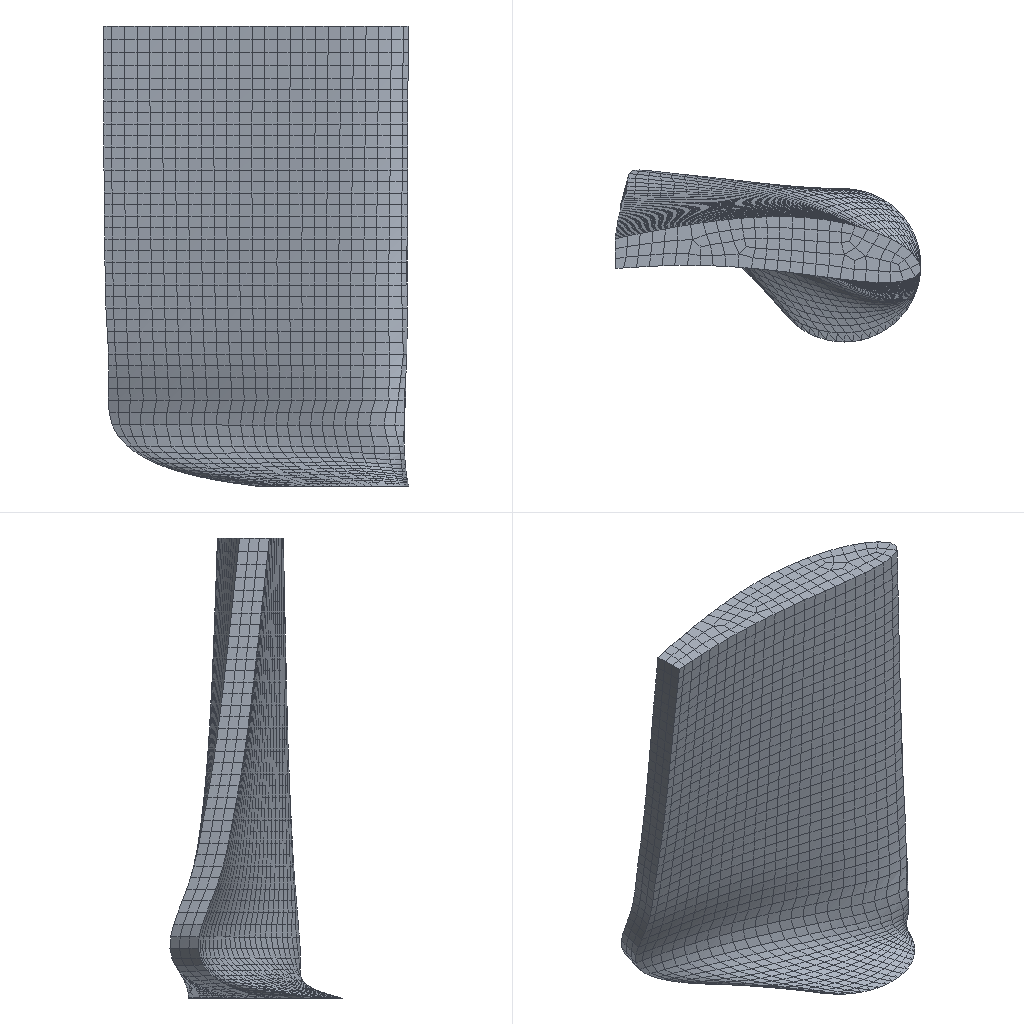Simulation study | abaqus
Set-up summary:
category,name,step,type,value,unit,region
solver,abaqus,,Abaqus/CAE 2024
units,SI m-kg-s (Pa),,inferred,E=1.5e+10 density=900
analysis,Step-1,,dynamic explicit,nlgeom=True; time_period=2.218
mesh,nodes,,,6429
mesh,elements,,,4944
element_type,C3D8R,,,4944
material,WOOD,,E,1.5e+10
material,WOOD,,nu,0.3
material,WOOD,,density,900
material,WOOD,,behaviors,damping
section,WOOD,,solid section,,,Set-1
load,Q1,Step-1,concentrated force,"1 [dir=(1, 0, 0)]",,Set-1
load,Q2,Step-1,concentrated force,"1 [dir=(1, 0, 0)]",,Set-2
load,Q3,Step-1,concentrated force,"1 [dir=(1, 0, 0)]",,Set-3
load,Q4,Step-1,concentrated force,"1 [dir=(1, 0, 0)]",,Set-4
load,Q5,Step-1,concentrated force,"1 [dir=(1, 0, 0)]",,Set-5
load,Q6,Step-1,concentrated force,"1 [dir=(1, 0, 0)]",,Set-6
load,Q7,Step-1,concentrated force,"1 [dir=(1, 0, 0)]",,Set-7
load,Q8,Step-1,concentrated force,"1 [dir=(1, 0, 0)]",,Set-8
load,Q9,Step-1,concentrated force,"1 [dir=(1, 0, 0)]",,Set-9
load,Q10,Step-1,concentrated force,"1 [dir=(1, 0, 0)]",,Set-10
load,Z1,Step-1,concentrated force,"1 [dir=(0, 1, 0)]",,Set-1
load,Z2,Step-1,concentrated force,"1 [dir=(0, 1, 0)]",,Set-2
load,Z3,Step-1,concentrated force,"1 [dir=(0, 1, 0)]",,Set-3
load,Z4,Step-1,concentrated force,"1 [dir=(0, 1, 0)]",,Set-4
load,Z5,Step-1,concentrated force,"1 [dir=(0, 1, 0)]",,Set-5
load,Z6,Step-1,concentrated force,"1 [dir=(0, 1, 0)]",,Set-6
load,Z7,Step-1,concentrated force,"1 [dir=(0, 1, 0)]",,Set-7
load,Z8,Step-1,concentrated force,"1 [dir=(0, 1, 0)]",,Set-8
load,Z9,Step-1,concentrated force,"1 [dir=(0, 1, 0)]",,Set-9
load,Z10,Step-1,concentrated force,"1 [dir=(0, 1, 0)]",,Set-10
bc,BC-1,Step-1,encastre,[dofs=ENCASTRE],,_PickedSet47
Abaqus input file, long lists of numbers shortened, first 290 of 1023 lines:
*Heading
** Job name: deck Model name: Model-1-Copy-Copy
** Generated by: Abaqus/CAE 2024
*Preprint, echo=NO, model=NO, history=NO, contact=NO
**
** PARTS
**
*Part, name=P16CMblade-Copy
*End Part
**
**
** ASSEMBLY
**
*Assembly, name=Assembly
**
*Instance, name=P16CMblade-Copy-1, part=P16CMblade-Copy
*Node
      1, -0.3723,  0.05119,  0.8526
      2, -0.3725, 0.002756,  0.8526
** (6417 more lines like these left out)
*Element, type=C3D8R
  1,    2,   26,  671,   27,   77,  975, 3494,  874
  2,   75,  698,  744,   76,  826, 3521, 3567,  825
** (4942 more lines like these left out)
*Nset, nset=Set-1, generate
    1,  6419,     1
*Elset, elset=Set-1, generate
    1,  4944,     1
** Section: Section-1
*Solid Section, elset=Set-1, material=WOOD
,
*End Instance
**
*Node
      1, -0.06243, 0.04167,  0.2223
*Node
      2, -0.09256, 0.05414,  0.2991
*Node
      3, -0.09701, 0.04794,  0.3745
*Node
      4, -0.1035, 0.045,  0.4497
*Node
      5, -0.108, 0.04136,  0.5244
*Node
      6, -0.1074,  0.03725,  0.6
*Node
      7, -0.106, 0.03382,  0.6742
*Node
      8, -0.1069, 0.03147,  0.7492
*Node
      9, -0.1111, 0.02943,  0.8249
*Node
     10, -0.1145, 0.02727,  0.8996
*Nset, nset=Set-1, instance=P16CMblade-Copy-1
 2706,
*Nset, nset=Set-2, instance=P16CMblade-Copy-1
 2423,
*Nset, nset=Set-3, instance=P16CMblade-Copy-1
 2190,
*Nset, nset=Set-4, instance=P16CMblade-Copy-1
 1957,
*Nset, nset=Set-5, instance=P16CMblade-Copy-1
 1725,
*Nset, nset=Set-6, instance=P16CMblade-Copy-1
 1535,
*Nset, nset=Set-7, instance=P16CMblade-Copy-1
 4057,
*Nset, nset=Set-8, instance=P16CMblade-Copy-1
 1119,
*Nset, nset=Set-9, instance=P16CMblade-Copy-1
 3595,
*Nset, nset=Set-10, instance=P16CMblade-Copy-1
 3376,
*Nset, nset=_PickedSet47, internal, instance=P16CMblade-Copy-1
   19,   20,   21,   22,  552,  553,  554,  555,  556,  557,  558,  559,  560,  561,  562,  563
  564,  565,  566,  567,  568,  569,  570,  571,  572,  573,  574,  575,  576,  577,  578,  579
** (7 more lines like these left out)
*Elset, elset=_PickedSet47, internal, instance=P16CMblade-Copy-1, generate
 4430,  4532,     1
*End Assembly
*Amplitude, name=Q1
          0.001,     0.0008927,           0.002,    -10.208,           0.003,    -15.004,           0.004,    -14.992
          0.005,    -14.896,           0.006,    -14.758,           0.007,    -14.573,           0.008,    -14.344
          0.009,    -14.078,            0.01,    -13.783,           0.011,    -13.456,           0.012,       -13.104
          0.013,    -12.739,           0.014,    -12.363,           0.015,    -11.999,           0.016,    -11.648
          0.017,    -11.318,           0.018,    -10.972,           0.019,    -10.59,            0.02,    -10.166
          0.021,    -9.717,           0.022,    -9.265,           0.023,    -8.835,           0.024,    -8.422
          0.025,    -8.028,           0.026,    -7.64,           0.027,    -7.247,           0.028,    -6.843
          0.029,    -6.429,            0.03,    -6.017,           0.031,    -5.621,           0.032,    -5.255
          0.033,    -4.946,           0.034,        -4.699,           0.035,    -4.522,           0.036,    -4.407
          0.037,    -4.336,           0.038,       -4.284,           0.039,    -4.228,            0.04,    -4.158
          0.041,    -4.061,           0.042,    -3.941,           0.043,    -3.805,           0.044,    -3.664
          0.045,    -3.439,           0.046,    -3.417,           0.047,         -3.45,           0.048,    -3.538
          0.049,    -3.663,            0.05,       -3.821,           0.051,       -4.012,           0.052,    -4.231
          0.053,    -4.472,           0.054,    -4.724,           0.055,    -4.957,           0.056,    -5.158
          0.057,    -5.33,           0.058,    -5.464,           0.059,    -5.548,            0.06,        -5.586
          0.061,    -5.589,           0.062,        -5.557,           0.063,    -5.501,           0.064,    -5.431
          0.065,    -5.347,           0.066,    -5.25,           0.067,    -5.13,           0.068,    -4.986
          0.069,    -4.816,            0.07,    -4.623,           0.071,    -4.417,           0.072,       -4.213
          0.073,    -4.034,           0.074,    -3.895,           0.075,    -3.803,           0.076,    -3.761
          0.077,    -3.761,           0.078,    -3.785,           0.079,    -3.831,            0.08,    -3.893
          0.081,    -3.96,           0.082,    -4.025,           0.083,    -4.081,           0.084,    -4.123
          0.085,        -4.149,           0.086,       -4.165,           0.087,    -4.17,           0.088,    -4.169
          0.089,       -4.161,            0.09,    -4.144,           0.091,    -4.125,           0.092,    -4.095
          0.093,    -4.052,           0.094,    -4.,           0.095,    -3.945,           0.096,    -3.889
          0.097,    -3.832,           0.098,    -3.771,           0.099,    -3.714,             0.1,    -3.66
          0.101,    -3.613,           0.102,    -3.572,           0.103,    -3.537,           0.104,    -3.506
          0.105,    -3.478,           0.106,    -3.451,           0.107,    -3.426,           0.108,       -3.403
          0.109,    -3.381,            0.11,    -3.364,           0.111,    -3.348,           0.112,    -3.333
          0.113,    -3.317,           0.114,    -3.3,           0.115,    -3.282,           0.116,       -3.263
          0.117,    -3.245,           0.118,    -3.227,           0.119,       -3.209,            0.12,    -3.191
          0.121,    -3.172,           0.122,       -3.152,           0.123,    -3.133,           0.124,    -3.114
          0.125,    -3.097,           0.126,    -3.082,           0.127,    -3.069,           0.128,       -3.059
          0.129,    -3.05,            0.13,    -3.043,           0.131,    -3.038,           0.132,    -3.035
          0.133,    -3.033,           0.134,    -3.034,           0.135,    -3.036,           0.136,    -3.038
          0.137,    -3.041,           0.138,    -3.042,           0.139,    -3.043,            0.14,    -3.04
          0.141,       -3.035,           0.142,    -3.03,           0.143,    -3.023,           0.144,    -3.016
          0.145,    -3.01,           0.146,    -3.005,           0.147,       -3.002,           0.148,    -3.001
          0.149,    -3.,            0.15,       -2.998,           0.151,    -2.995,           0.152,    -2.989
          0.153,    -2.98,           0.154,        -2.971,           0.155,    -2.962,           0.156,    -2.956
          0.157,    -2.952,           0.158,    -2.952,           0.159,    -2.954,            0.16,    -2.958
** (515 more lines like these left out)
*Amplitude, name=Q2
          0.001,      2.0276e-05,           0.002,        1.997,           0.003,     1.898,           0.004,     1.983
          0.005,        2.059,           0.006,        2.213,           0.007,     2.371,           0.008,     2.55
          0.009,        2.74,            0.01,     2.942,           0.011,     3.163,           0.012,     3.395
          0.013,     3.636,           0.014,         3.904,           0.015,     4.219,           0.016,     4.581
          0.017,     4.972,           0.018,     5.397,           0.019,     5.84,            0.02,         6.278
          0.021,     6.698,           0.022,     7.105,           0.023,         7.505,           0.024,     7.916
          0.025,     8.336,           0.026,     8.773,           0.027,     9.226,           0.028,         9.695
          0.029,     10.182,            0.03,     10.673,           0.031,     11.148,           0.032,     11.569
          0.033,        11.887,           0.034,     12.064,           0.035,     12.1,           0.036,     12.027
          0.037,     11.9,           0.038,     11.78,           0.039,     11.699,            0.04,     11.673
          0.041,     11.705,           0.042,        11.789,           0.043,        11.908,           0.044,     12.044
          0.045,        12.281,           0.046,     12.357,           0.047,     12.384,           0.048,     12.374
          0.049,        12.334,            0.05,        12.269,           0.051,     12.18,           0.052,     12.065
          0.053,     11.93,           0.054,     11.787,           0.055,     11.646,           0.056,        11.499
          0.057,     11.335,           0.058,        11.135,           0.059,     10.892,            0.06,     10.614
          0.061,     10.314,           0.062,        10.021,           0.063,     9.763,           0.064,         9.546
          0.065,     9.363,           0.066,     9.198,           0.067,         9.035,           0.068,         8.861
          0.069,         8.676,            0.07,     8.484,           0.071,     8.298,           0.072,         8.127
          0.073,         7.981,           0.074,     7.868,           0.075,     7.791,           0.076,         7.755
          0.077,         7.742,           0.078,     7.739,           0.079,     7.725,            0.08,     7.684
          0.081,     7.61,           0.082,     7.499,           0.083,     7.358,           0.084,         7.19
          0.085,         7.003,           0.086,     6.793,           0.087,     6.569,           0.088,     6.349
          0.089,         6.142,            0.09,     5.965,           0.091,     5.816,           0.092,     5.701
          0.093,     5.613,           0.094,     5.534,           0.095,     5.468,           0.096,     5.411
          0.097,     5.365,           0.098,         5.321,           0.099,     5.277,             0.1,         5.232
          0.101,     5.182,           0.102,     5.127,           0.103,     5.067,           0.104,         5.003
          0.105,         4.938,           0.106,     4.875,           0.107,     4.813,           0.108,     4.753
          0.109,     4.699,            0.11,     4.648,           0.111,     4.602,           0.112,          4.561
          0.113,     4.522,           0.114,     4.484,           0.115,     4.445,           0.116,     4.404
          0.117,         4.361,           0.118,         4.318,           0.119,     4.275,            0.12,     4.234
          0.121,     4.196,           0.122,     4.161,           0.123,     4.128,           0.124,     4.097
          0.125,     4.066,           0.126,         4.034,           0.127,          4.,           0.128,         3.965
          0.129,     3.928,            0.13,         3.892,           0.131,         3.858,           0.132,     3.826
          0.133,     3.797,           0.134,     3.773,           0.135,     3.751,           0.136,     3.731
          0.137,     3.711,           0.138,     3.689,           0.139,     3.666,            0.14,     3.641
          0.141,     3.617,           0.142,          3.593,           0.143,     3.571,           0.144,         3.551
          0.145,     3.533,           0.146,     3.517,           0.147,     3.502,           0.148,     3.487
          0.149,     3.47,            0.15,     3.45,           0.151,     3.428,           0.152,     3.402
          0.153,         3.374,           0.154,         3.346,           0.155,     3.318,           0.156,     3.291
          0.157,     3.266,           0.158,     3.243,           0.159,     3.221,            0.16,     3.201
** (515 more lines like these left out)
*Amplitude, name=Q3
          0.001,     2.06759e-05,           0.002,     2.03,           0.003,     1.928,           0.004,     1.994
          0.005,     2.056,           0.006,       2.194,           0.007,     2.337,           0.008,       2.516
          0.009,     2.716,            0.01,     2.941,           0.011,     3.168,           0.012,        3.356
          0.013,     3.542,           0.014,        3.775,           0.015,        4.057,           0.016,     4.346
          0.017,     4.639,           0.018,     4.966,           0.019,        5.328,            0.02,     5.727
          0.021,     6.16,           0.022,     6.622,           0.023,        7.102,           0.024,     7.594
          0.025,        8.082,           0.026,     8.571,           0.027,        9.059,           0.028,     9.553
          0.029,       10.06,            0.03,     10.575,           0.031,        11.076,           0.032,          11.544
          0.033,     11.939,           0.034,       12.215,           0.035,       12.343,           0.036,       12.33
          0.037,     12.211,           0.038,       12.039,           0.039,     11.87,            0.04,     11.745
          0.041,     11.674,           0.042,       11.661,           0.043,       11.695,           0.044,       11.758
          0.045,       11.901,           0.046,       11.959,           0.047,     11.985,           0.048,       11.985
          0.049,     11.96,            0.05,       11.909,           0.051,       11.838,           0.052,       11.751
          0.053,       11.656,           0.054,       11.558,           0.055,     11.45,           0.056,     11.302
          0.057,       11.091,           0.058,     10.817,           0.059,     10.509,            0.06,       10.205
          0.061,     9.918,           0.062,     9.654,           0.063,     9.409,           0.064,     9.179
          0.065,        8.961,           0.066,     8.744,           0.067,     8.52,           0.068,     8.286
          0.069,     8.044,            0.07,     7.803,           0.071,        7.571,           0.072,     7.359
          0.073,     7.185,           0.074,     7.068,           0.075,        7.01,           0.076,        7.008
          0.077,     7.051,           0.078,     7.127,           0.079,        7.209,            0.08,     7.271
          0.081,     7.294,           0.082,        7.257,           0.083,     7.163,           0.084,     7.02
          0.085,     6.832,           0.086,        6.611,           0.087,     6.371,           0.088,         6.122
          0.089,     5.878,            0.09,     5.655,           0.091,         5.461,           0.092,     5.307
          0.093,     5.194,           0.094,         5.115,           0.095,     5.071,           0.096,     5.039
          0.097,     5.013,           0.098,     4.981,           0.099,     4.944,             0.1,     4.9
          0.101,     4.846,           0.102,     4.779,           0.103,     4.706,           0.104,        4.632
          0.105,     4.56,           0.106,        4.492,           0.107,     4.428,           0.108,         4.367
          0.109,        4.312,            0.11,        4.262,           0.111,     4.216,           0.112,        4.172
          0.113,     4.13,           0.114,         4.087,           0.115,        4.045,           0.116,     4.003
          0.117,        3.964,           0.118,     3.928,           0.119,        3.896,            0.12,     3.867
          0.121,        3.84,           0.122,     3.814,           0.123,     3.787,           0.124,     3.758
          0.125,     3.727,           0.126,     3.695,           0.127,           3.662,           0.128,     3.629
          0.129,     3.598,            0.13,     3.569,           0.131,     3.544,           0.132,     3.52
          0.133,     3.498,           0.134,     3.476,           0.135,     3.454,           0.136,     3.431
          0.137,        3.407,           0.138,        3.383,           0.139,     3.359,            0.14,     3.335
          0.141,     3.313,           0.142,     3.292,           0.143,        3.272,           0.144,     3.255
          0.145,     3.238,           0.146,         3.222,           0.147,     3.205,           0.148,     3.188
          0.149,        3.169,            0.15,        3.149,           0.151,     3.128,           0.152,         3.107
          0.153,     3.085,           0.154,     3.062,           0.155,     3.04,           0.156,     3.018
          0.157,         2.997,           0.158,        2.976,           0.159,        2.956,            0.16,     2.937
** (515 more lines like these left out)
*Amplitude, name=Q4
          0.001,     8.10815e-06,           0.002,     1.453,           0.003,     1.449,           0.004,     1.508
          0.005,     1.538,           0.006,     1.633,           0.007,     1.738,           0.008,     1.877
          0.009,     2.048,            0.01,         2.246,           0.011,     2.464,           0.012,     2.644
          0.013,     2.794,           0.014,     2.978,           0.015,     3.239,           0.016,     3.479
          0.017,     3.687,           0.018,         3.876,           0.019,     4.058,            0.02,         4.242
          0.021,     4.416,           0.022,     4.612,           0.023,     4.848,           0.024,     5.155
          0.025,     5.543,           0.026,         6.016,           0.027,     6.556,           0.028,     7.146
          0.029,     7.781,            0.03,     8.443,           0.031,     9.106,           0.032,     9.733
          0.033,        10.253,           0.034,     10.625,           0.035,     10.832,           0.036,     10.909
          0.037,        10.91,           0.038,     10.89,           0.039,     10.884,            0.04,     10.915
          0.041,         10.973,           0.042,     11.052,           0.043,     11.138,           0.044,        11.219
          0.045,     11.307,           0.046,     11.307,           0.047,     11.269,           0.048,     11.202
          0.049,     11.11,            0.05,     11.001,           0.051,     10.88,           0.052,     10.751
          0.053,     10.618,           0.054,     10.481,           0.055,     10.334,           0.056,     10.159
          0.057,     9.945,           0.058,     9.687,           0.059,     9.403,            0.06,     9.12
          0.061,     8.847,           0.062,     8.588,           0.063,     8.346,           0.064,     8.12
          0.065,     7.911,           0.066,     7.719,           0.067,     7.539,           0.068,     7.369
          0.069,     7.206,            0.07,     7.045,           0.071,     6.875,           0.072,     6.692
          0.073,     6.503,           0.074,     6.343,           0.075,         6.258,           0.076,     6.263
          0.077,     6.321,           0.078,     6.385,           0.079,     6.434,            0.08,     6.466
          0.081,     6.479,           0.082,     6.447,           0.083,     6.36,           0.084,     6.231
          0.085,         6.076,           0.086,     5.903,           0.087,     5.727,           0.088,     5.559
          0.089,     5.403,            0.09,     5.267,           0.091,     5.148,           0.092,     5.046
          0.093,     4.964,           0.094,     4.895,           0.095,     4.838,           0.096,     4.786
          0.097,     4.738,           0.098,     4.686,           0.099,     4.631,             0.1,     4.571
          0.101,     4.506,           0.102,         4.433,           0.103,     4.358,           0.104,     4.283
          0.105,     4.21,           0.106,     4.141,           0.107,     4.078,           0.108,     4.017
          0.109,     3.96,            0.11,     3.905,           0.111,     3.855,           0.112,     3.809
          0.113,     3.767,           0.114,     3.73,           0.115,     3.699,           0.116,     3.671
          0.117,     3.647,           0.118,     3.626,           0.119,     3.606,            0.12,     3.586
          0.121,     3.565,           0.122,     3.543,           0.123,     3.521,           0.124,     3.498
          0.125,     3.475,           0.126,     3.452,           0.127,     3.43,           0.128,     3.408
          0.129,     3.386,            0.13,     3.365,           0.131,     3.342,           0.132,     3.319
          0.133,         3.296,           0.134,         3.273,           0.135,     3.25,           0.136,     3.227
          0.137,     3.206,           0.138,     3.184,           0.139,     3.164,            0.14,     3.143
          0.141,     3.124,           0.142,     3.104,           0.143,     3.086,           0.144,     3.068
          0.145,         3.051,           0.146,     3.034,           0.147,     3.017,           0.148,          2.999
          0.149,     2.981,            0.15,     2.962,           0.151,     2.943,           0.152,     2.923
          0.153,     2.903,           0.154,     2.883,           0.155,     2.863,           0.156,     2.843
          0.157,     2.824,           0.158,     2.804,           0.159,     2.785,            0.16,     2.765
** (515 more lines like these left out)
*Amplitude, name=Q5
          0.001,     5.66292e-06,           0.002,     1.283,           0.003,     1.307,           0.004,     1.358
          0.005,     1.374,           0.006,     1.431,           0.007,     1.488,           0.008,      1.573
          0.009,     1.694,            0.01,     1.85,           0.011,     2.034,           0.012,     2.172
          0.013,     2.284,           0.014,     2.446,           0.015,     2.674,           0.016,      2.895
          0.017,     3.074,           0.018,      3.227,           0.019,     3.357,            0.02,     3.476
          0.021,     3.585,           0.022,     3.692,           0.023,     3.805,           0.024,         3.934
          0.025,     4.087,           0.026,      4.268,           0.027,      4.476,           0.028,     4.724
          0.029,     5.012,            0.03,     5.34,           0.031,     5.701,           0.032,     6.089
          0.033,     6.482,           0.034,     6.855,           0.035,     7.185,           0.036,     7.467
          0.037,     7.716,           0.038,     7.946,           0.039,      8.179,            0.04,     8.43
          0.041,     8.689,           0.042,     8.948,           0.043,     9.197,           0.044,     9.416
          0.045,      9.714,           0.046,      9.791,           0.047,     9.817,           0.048,      9.801
          0.049,     9.749,            0.05,     9.662,           0.051,     9.548,           0.052,         9.41
          0.053,     9.258,           0.054,     9.095,           0.055,     8.927,           0.056,     8.751
          0.057,      8.564,           0.058,     8.361,           0.059,     8.146,            0.06,     7.929
          0.061,     7.718,           0.062,     7.517,           0.063,         7.334,           0.064,     7.167
          0.065,     7.017,           0.066,     6.883,           0.067,     6.76,           0.068,     6.642
          0.069,     6.527,            0.07,     6.413,           0.071,     6.297,           0.072,     6.181
          0.073,     6.076,           0.074,     5.993,           0.075,     5.929,           0.076,     5.879
          0.077,     5.833,           0.078,      5.788,           0.079,     5.745,            0.08,     5.694
          0.081,     5.625,           0.082,     5.531,           0.083,     5.416,           0.084,     5.288
          0.085,      5.156,           0.086,     5.028,           0.087,     4.914,           0.088,     4.815
          0.089,     4.732,            0.09,     4.662,           0.091,     4.604,           0.092,     4.557
          0.093,     4.519,           0.094,         4.486,           0.095,     4.452,           0.096,     4.413
          0.097,          4.368,           0.098,     4.315,           0.099,     4.257,             0.1,     4.195
          0.101,     4.132,           0.102,     4.066,           0.103,     3.999,           0.104,     3.93
          0.105,     3.86,           0.106,     3.788,           0.107,     3.716,           0.108,     3.649
          0.109,     3.59,            0.11,     3.539,           0.111,         3.497,           0.112,     3.462
          0.113,     3.435,           0.114,     3.414,           0.115,     3.399,           0.116,     3.386
          0.117,     3.375,           0.118,     3.365,           0.119,     3.355,            0.12,      3.346
          0.121,     3.336,           0.122,     3.326,           0.123,     3.315,           0.124,     3.302
          0.125,     3.287,           0.126,         3.27,           0.127,     3.25,           0.128,     3.229
          0.129,     3.206,            0.13,     3.182,           0.131,     3.158,           0.132,      3.134
          0.133,     3.11,           0.134,     3.087,           0.135,     3.063,           0.136,     3.039
          0.137,     3.016,           0.138,     2.992,           0.139,     2.969,            0.14,     2.948
          0.141,     2.928,           0.142,      2.909,           0.143,         2.891,           0.144,     2.874
          0.145,     2.857,           0.146,     2.839,           0.147,     2.822,           0.148,     2.803
          0.149,     2.785,            0.15,     2.766,           0.151,     2.748,           0.152,     2.73
          0.153,          2.712,           0.154,     2.694,           0.155,     2.675,           0.156,     2.656
          0.157,     2.636,           0.158,     2.615,           0.159,     2.594,            0.16,     2.574
** (515 more lines like these left out)
Last 497 lines:
          0.101,        5.482,           0.102,        5.411,           0.103,        5.346,           0.104,        5.287
          0.105,        5.234,           0.106,        5.186,           0.107,         5.142,           0.108,        5.098
          0.109,        5.054,            0.11,        5.009,           0.111,        4.962,           0.112,        4.915
          0.113,         4.866,           0.114,        4.818,           0.115,        4.771,           0.116,        4.724
          0.117,        4.678,           0.118,        4.632,           0.119,        4.587,            0.12,        4.543
          0.121,        4.5,           0.122,        4.459,           0.123,        4.418,           0.124,         4.377
          0.125,        4.337,           0.126,        4.296,           0.127,        4.256,           0.128,        4.215
          0.129,        4.175,            0.13,        4.136,           0.131,          4.098,           0.132,        4.062
          0.133,         4.028,           0.134,        3.996,           0.135,        3.968,           0.136,        3.944
          0.137,        3.923,           0.138,        3.905,           0.139,        3.889,            0.14,        3.876
          0.141,        3.865,           0.142,        3.857,           0.143,        3.852,           0.144,        3.849
          0.145,        3.849,           0.146,         3.85,           0.147,        3.851,           0.148,        3.85
          0.149,        3.846,            0.15,         3.837,           0.151,        3.822,           0.152,        3.802
          0.153,        3.775,           0.154,        3.745,           0.155,         3.711,           0.156,        3.677
          0.157,        3.644,           0.158,        3.613,           0.159,        3.584,            0.16,        3.558
** (515 more lines like these left out)
*Amplitude, name=Z2
             0.,     2.57247e-07,           0.001,        2.638,           0.002,        2.523,           0.003,        2.755
          0.004,        2.977,           0.005,        3.378,           0.006,        3.799,           0.007,        4.261
          0.008,        4.73,     0.009,        5.189,            0.01,        5.645,           0.011,         6.077
          0.012,         6.477,           0.013,         6.864,           0.014,        7.265,           0.015,        7.661
          0.016,          8.051,           0.017,         8.468,           0.018,        8.914,           0.019,        9.391
           0.02,        9.883,           0.021,        10.382,           0.022,        10.871,           0.023,        11.355
          0.024,        11.824,           0.025,        12.281,           0.026,        12.721,           0.027,        13.139
          0.028,        13.548,           0.029,        13.955,            0.03,        14.357,           0.031,        14.74
          0.032,        15.067,           0.033,        15.304,           0.034,        15.434,           0.035,        15.467
          0.036,        15.443,           0.037,        15.422,           0.038,        15.451,           0.039,        15.561
           0.04,        15.758,           0.041,        16.036,           0.042,        16.368,           0.043,        16.733
          0.045,        17.419,           0.046,        17.7,           0.047,        17.896,           0.048,        18.021
          0.049,        18.09,            0.05,        18.113,           0.051,        18.097,           0.052,        18.049
          0.053,        17.978,      0.054,        17.896,           0.055,         17.817,           0.056,        17.727
          0.057,        17.61,      0.058,        17.448,           0.059,         17.23,            0.06,        16.966
          0.061,        16.652,      0.062,        16.31,      0.063,         15.972,           0.064,        15.664
     0.065,        15.4,      0.066,         15.171,           0.067,         14.953,           0.068,        14.719
     0.069,        14.465,      0.07,         14.187,           0.071,        13.89,           0.072,        13.589
     0.073,        13.305,           0.074,        13.061,           0.075,         12.866,      0.076,        12.726
     0.077,        12.63,      0.078,        12.568,           0.079,        12.516,      0.08,        12.456
          0.081,        12.378,           0.082,        12.263,           0.083,         12.111,      0.084,        11.92
     0.085,        11.692,      0.086,        11.416,           0.087,        11.105,      0.088,        10.787
          0.089,        10.478,            0.09,        10.198,      0.091,        9.964,      0.092,        9.783
     0.093,        9.651,           0.094,         9.547,      0.095,        9.465,           0.096,        9.391
          0.097,        9.32,           0.098,        9.246,      0.099,        9.166,             0.1,        9.077
          0.101,        8.979,           0.102,        8.869,           0.103,         8.757,           0.104,        8.644
          0.105,        8.534,           0.106,        8.425,           0.107,        8.323,           0.108,        8.225
          0.109,        8.137,            0.11,        8.059,           0.111,        7.987,           0.112,        7.921
          0.113,        7.857,           0.114,        7.793,           0.115,        7.728,           0.116,        7.659
          0.117,        7.587,           0.118,        7.513,           0.119,         7.439,            0.12,        7.367
          0.121,        7.299,           0.122,        7.235,           0.123,        7.175,           0.124,         7.118
          0.125,        7.063,           0.126,        7.007,           0.127,        6.95,           0.128,        6.891
          0.129,        6.83,            0.13,        6.769,           0.131,        6.711,           0.132,        6.656
          0.133,        6.606,           0.134,        6.561,           0.135,        6.523,           0.136,        6.488
          0.137,        6.458,           0.138,        6.427,           0.139,         6.398,            0.14,        6.369
          0.141,        6.341,           0.142,        6.315,           0.143,        6.292,           0.144,        6.273
          0.145,        6.258,           0.146,        6.246,           0.147,        6.237,           0.148,         6.227
          0.149,        6.215,            0.15,        6.199,           0.151,        6.178,           0.152,         6.152
          0.153,        6.122,           0.154,        6.088,           0.155,        6.053,           0.156,        6.018
          0.157,        5.984,           0.158,        5.952,           0.159,        5.922,            0.16,        5.894
** (515 more lines like these left out)
*Amplitude, name=Z3
             0.,    -1.10892e-06,           0.001,        3.343,           0.002,        3.065,           0.003,         3.216
          0.004,        3.369,           0.005,          3.748,           0.006,        4.165,           0.007,        4.654
          0.008,        5.168,     0.009,        5.687,            0.01,        6.192,           0.011,        6.592
          0.012,        6.878,           0.013,        7.123,           0.014,        7.415,           0.015,        7.763
          0.016,        8.195,           0.017,         8.743,           0.018,        9.354,           0.019,        10.003
           0.02,        10.653,           0.021,        11.28,           0.022,        11.866,           0.023,        12.413
          0.024,         12.924,           0.025,        13.414,           0.026,          13.891,           0.027,        14.373
          0.028,         14.876,           0.029,         15.406,            0.03,        15.963,           0.031,        16.533
          0.032,        17.071,           0.033,         17.522,           0.034,        17.837,           0.035,        17.997
          0.036,        18.025,           0.037,        17.972,           0.038,        17.904,           0.039,         17.874
           0.04,        17.908,           0.041,        18.023,           0.042,        18.212,           0.043,        18.46
          0.045,        19.033,           0.046,        19.334,           0.047,        19.589,           0.048,        19.802
          0.049,        19.976,            0.05,        20.112,           0.051,        20.215,           0.052,         20.295
          0.053,        20.366,      0.054,        20.434,           0.055,         20.486,           0.056,        20.472
          0.057,        20.339,      0.058,        20.066,           0.059,        19.688,            0.06,         19.269
          0.061,        18.85,      0.062,        18.458,      0.063,        18.106,           0.064,         17.79
     0.065,        17.493,      0.066,        17.188,           0.067,        16.844,           0.068,        16.443
     0.069,        15.989,      0.07,        15.498,           0.071,        15.003,           0.072,        14.554
     0.073,        14.2,           0.074,         13.978,           0.075,         13.892,      0.076,        13.932
     0.077,        14.054,      0.078,        14.22,           0.079,        14.374,      0.08,        14.485
          0.081,        14.536,           0.082,        14.505,           0.083,        14.387,      0.084,        14.188
     0.085,        13.905,      0.086,        13.545,           0.087,         13.134,      0.088,        12.689
          0.089,        12.244,            0.09,        11.832,      0.091,        11.461,      0.092,        11.154
     0.093,        10.91,           0.094,        10.723,      0.095,         10.591,           0.096,        10.482
          0.097,         10.393,           0.098,        10.31,      0.099,        10.228,             0.1,        10.143
          0.101,        10.051,           0.102,         9.934,           0.103,        9.804,           0.104,        9.662
          0.105,        9.52,           0.106,        9.378,           0.107,        9.245,           0.108,         9.119
          0.109,        9.007,            0.11,        8.906,           0.111,        8.811,           0.112,        8.72
          0.113,        8.629,           0.114,        8.54,           0.115,        8.451,           0.116,        8.365
          0.117,        8.283,           0.118,        8.208,           0.119,        8.141,            0.12,        8.08
          0.121,        8.026,           0.122,        7.974,           0.123,        7.921,           0.124,        7.866
          0.125,        7.807,           0.126,        7.744,           0.127,        7.678,           0.128,        7.613
          0.129,        7.551,            0.13,        7.496,           0.131,        7.448,           0.132,        7.407
          0.133,        7.371,           0.134,        7.339,           0.135,        7.307,           0.136,          7.274
          0.137,        7.24,           0.138,        7.202,           0.139,        7.163,            0.14,        7.126
          0.141,        7.091,           0.142,        7.061,           0.143,        7.036,           0.144,         7.015
          0.145,        6.999,           0.146,        6.985,           0.147,        6.971,           0.148,         6.956
          0.149,        6.937,            0.15,        6.915,           0.151,        6.89,           0.152,        6.861
          0.153,        6.83,           0.154,        6.798,           0.155,        6.766,           0.156,        6.735
          0.157,        6.706,           0.158,        6.678,           0.159,        6.651,            0.16,         6.625
** (515 more lines like these left out)
*Amplitude, name=Z4
             0.,     1.23106e-06,           0.001,        3.872,           0.002,        3.514,           0.003,        3.651
          0.004,        3.774,           0.005,        4.145,           0.006,        4.557,           0.007,        5.064
          0.008,        5.62,     0.009,        6.189,            0.01,        6.771,           0.011,        7.258
          0.012,        7.604,           0.013,        7.862,           0.014,        8.126,           0.015,        8.397
          0.016,        8.744,           0.017,        9.254,           0.018,          9.863,           0.019,        10.525
           0.02,        11.175,           0.021,        11.775,           0.022,         12.325,           0.023,        12.856
          0.024,        13.4,           0.025,        13.98,           0.026,        14.59,           0.027,        15.242
          0.028,        15.942,           0.029,        16.686,            0.03,        17.47,           0.031,        18.274
          0.032,        19.032,           0.033,        19.684,           0.034,        20.183,           0.035,         20.528
          0.036,        20.754,           0.037,        20.922,           0.038,        21.088,           0.039,        21.292
           0.04,        21.538,           0.041,        21.832,           0.042,        22.163,           0.043,        22.512
          0.045,        23.159,           0.046,        23.43,           0.047,        23.624,           0.048,        23.748
          0.049,        23.815,            0.05,        23.838,           0.051,        23.829,           0.052,        23.804
          0.053,        23.777,      0.054,        23.744,           0.055,        23.687,           0.056,        23.556
          0.057,        23.306,      0.058,        22.919,           0.059,        22.422,            0.06,        21.863
          0.061,        21.276,      0.062,         20.691,      0.063,        20.127,           0.064,        19.605
     0.065,        19.141,      0.066,        18.741,           0.067,        18.399,           0.068,        18.099
     0.069,         17.842,      0.07,        17.609,           0.071,        17.383,           0.072,        17.138
     0.073,        16.878,           0.074,        16.669,           0.075,        16.557,      0.076,        16.576
     0.077,        16.677,      0.078,        16.829,           0.079,         16.963,      0.08,        17.049
          0.081,        17.049,           0.082,        16.944,           0.083,        16.721,      0.084,        16.399
     0.085,        16.004,      0.086,        15.557,           0.087,        15.091,      0.088,        14.646
          0.089,        14.221,            0.09,        13.856,      0.091,        13.53,      0.092,        13.253
     0.093,        13.029,           0.094,        12.826,      0.095,        12.659,           0.096,        12.502
          0.097,        12.358,           0.098,        12.216,      0.099,        12.078,             0.1,        11.939
          0.101,        11.802,           0.102,        11.659,           0.103,        11.517,           0.104,        11.377
          0.105,        11.24,           0.106,        11.104,           0.107,        10.969,           0.108,          10.833
          0.109,        10.701,            0.11,        10.573,           0.111,        10.447,           0.112,        10.323
          0.113,        10.203,           0.114,        10.092,           0.115,         9.99,           0.116,        9.897
          0.117,        9.814,           0.118,        9.74,           0.119,         9.672,            0.12,        9.609
          0.121,        9.548,           0.122,        9.487,           0.123,        9.425,           0.124,        9.363
          0.125,        9.301,           0.126,        9.241,           0.127,        9.183,           0.128,        9.13
          0.129,        9.08,            0.13,        9.034,           0.131,        8.99,           0.132,        8.948
          0.133,        8.907,           0.134,        8.865,           0.135,        8.823,           0.136,        8.781
          0.137,        8.739,           0.138,        8.696,           0.139,        8.656,            0.14,        8.618
          0.141,        8.583,           0.142,        8.551,           0.143,        8.523,           0.144,         8.498
          0.145,        8.475,           0.146,        8.453,           0.147,        8.432,           0.148,         8.409
          0.149,        8.384,            0.15,        8.357,           0.151,        8.327,           0.152,        8.297
          0.153,        8.265,           0.154,        8.234,           0.155,        8.204,           0.156,        8.175
          0.157,        8.147,           0.158,        8.119,           0.159,        8.09,            0.16,        8.06
** (515 more lines like these left out)
*Amplitude, name=Z5
             0.,    -2.04411e-07,           0.001,        4.064,           0.002,        3.704,           0.003,        3.839
          0.004,        3.948,           0.005,        4.302,           0.006,        4.697,           0.007,        5.189
          0.008,        5.756,     0.009,        6.355,            0.01,        6.981,           0.011,        7.513
          0.012,        7.887,           0.013,         8.158,           0.014,        8.401,           0.015,        8.636
          0.016,        8.946,           0.017,        9.438,           0.018,        10.061,           0.019,         10.762
           0.02,         11.452,           0.021,        12.077,           0.022,        12.612,           0.023,        13.075
          0.024,         13.511,           0.025,         13.949,           0.026,        14.414,           0.027,        14.935
          0.028,        15.527,           0.029,        16.188,            0.03,        16.906,           0.031,        17.664
          0.032,        18.401,           0.033,        19.06,           0.034,        19.593,           0.035,         19.99
          0.036,        20.289,           0.037,        20.542,           0.038,        20.815,           0.039,          21.155
           0.04,        21.564,           0.041,        22.042,           0.042,        22.569,           0.043,        23.109
          0.045,          24.102,           0.046,        24.527,           0.047,        24.865,           0.048,        25.123
          0.049,        25.3,            0.05,        25.395,           0.051,        25.411,           0.052,        25.357
          0.053,        25.25,      0.054,          25.093,           0.055,        24.899,           0.056,        24.654
          0.057,        24.35,      0.058,        23.984,           0.059,        23.579,            0.06,        23.164
          0.061,         22.749,      0.062,        22.352,      0.063,         21.971,           0.064,        21.603
     0.065,        21.238,      0.066,        20.889,           0.067,        20.547,           0.068,        20.219
     0.069,        19.909,      0.07,        19.609,           0.071,         19.31,           0.072,        19.032
     0.073,        18.793,           0.074,        18.639,           0.075,        18.594,      0.076,        18.647
     0.077,        18.738,      0.078,        18.822,           0.079,        18.849,      0.08,        18.789
          0.081,        18.634,           0.082,        18.365,           0.083,         18.003,      0.084,        17.569
     0.085,        17.109,      0.086,        16.644,           0.087,        16.22,      0.088,        15.845
          0.089,        15.527,            0.09,        15.256,      0.091,        15.026,      0.092,        14.823
     0.093,        14.653,           0.094,        14.49,      0.095,        14.342,           0.096,        14.195
          0.097,        14.045,           0.098,        13.889,      0.099,         13.729,             0.1,        13.564
          0.101,        13.399,           0.102,        13.23,           0.103,        13.066,           0.104,        12.907
          0.105,        12.753,           0.106,        12.603,           0.107,        12.452,           0.108,        12.297
          0.109,        12.142,            0.11,        11.992,           0.111,        11.846,           0.112,        11.707
          0.113,        11.578,           0.114,        11.462,           0.115,        11.356,           0.116,        11.261
          0.117,        11.175,           0.118,        11.097,           0.119,        11.027,            0.12,        10.964
          0.121,        10.907,           0.122,        10.854,           0.123,         10.805,           0.124,        10.757
          0.125,        10.709,           0.126,        10.662,           0.127,         10.614,           0.128,        10.566
          0.129,        10.519,            0.13,        10.472,           0.131,        10.427,           0.132,        10.382
          0.133,        10.337,           0.134,        10.292,           0.135,        10.247,           0.136,        10.2
          0.137,        10.153,           0.138,        10.106,           0.139,        10.061,            0.14,        10.019
          0.141,        9.982,           0.142,        9.948,           0.143,         9.919,           0.144,        9.892
          0.145,         9.867,           0.146,        9.841,           0.147,        9.813,           0.148,        9.785
          0.149,        9.755,            0.15,        9.724,           0.151,        9.694,           0.152,        9.664
          0.153,        9.635,           0.154,        9.607,           0.155,        9.577,           0.156,        9.547
          0.157,        9.515,           0.158,        9.481,           0.159,         9.446,            0.16,        9.411
** (515 more lines like these left out)
*Amplitude, name=Z6
             0.,    -2.87837e-08,           0.001,        4.195,           0.002,        3.8,           0.003,         3.918
          0.004,        4.001,           0.005,        4.32,           0.006,        4.695,           0.007,        5.148
          0.008,        5.693,     0.009,        6.273,            0.01,        6.888,           0.011,        7.458
          0.012,        7.872,           0.013,         8.15,           0.014,        8.397,           0.015,        8.589
          0.016,        8.828,           0.017,        9.229,           0.018,        9.793,           0.019,        10.463
           0.02,        11.156,           0.021,        11.806,           0.022,        12.383,           0.023,        12.896
          0.024,        13.385,           0.025,        13.879,           0.026,        14.386,           0.027,        14.924
          0.028,        15.516,           0.029,        16.164,            0.03,        16.862,           0.031,        17.586
          0.032,        18.248,           0.033,        18.76,           0.034,        19.051,           0.035,        19.1
          0.036,        18.959,           0.037,        18.747,           0.038,        18.596,           0.039,        18.614
           0.04,        18.85,           0.041,        19.292,           0.042,        19.894,           0.043,        20.587
          0.045,        21.999,           0.046,        22.649,           0.047,        23.207,           0.048,        23.671
          0.049,        24.036,            0.05,        24.304,           0.051,        24.482,           0.052,          24.562
          0.053,        24.561,      0.054,        24.476,           0.055,        24.322,           0.056,        24.1
          0.057,        23.806,      0.058,        23.435,           0.059,        23.003,            0.06,        22.542
          0.061,        22.079,      0.062,        21.648,      0.063,        21.277,           0.064,        20.972
     0.065,        20.739,      0.066,        20.571,           0.067,        20.459,           0.068,        20.391
     0.069,        20.353,      0.07,        20.337,           0.071,        20.33,           0.072,        20.329
     0.073,        20.327,           0.074,        20.322,           0.075,        20.315,      0.076,        20.295
     0.077,        20.245,      0.078,         20.149,           0.079,        19.987,      0.08,         19.747
          0.081,        19.438,           0.082,        19.06,           0.083,        18.637,      0.084,        18.201
     0.085,        17.785,      0.086,        17.405,           0.087,        17.084,      0.088,        16.812
          0.089,        16.579,            0.09,        16.374,      0.091,        16.192,      0.092,        16.033
     0.093,        15.904,           0.094,        15.794,      0.095,        15.699,           0.096,        15.601
          0.097,        15.489,           0.098,        15.355,      0.099,        15.199,             0.1,          15.023
          0.101,        14.83,           0.102,        14.623,           0.103,        14.413,           0.104,        14.206
          0.105,        14.006,           0.106,         13.817,           0.107,        13.636,           0.108,        13.465
          0.109,        13.306,            0.11,         13.157,           0.111,        13.015,           0.112,        12.877
          0.113,        12.747,           0.114,        12.627,           0.115,        12.516,           0.116,        12.418
          0.117,        12.333,           0.118,        12.261,           0.119,         12.201,            0.12,        12.152
          0.121,        12.111,           0.122,        12.075,           0.123,         12.039,           0.124,        12.004
          0.125,        11.967,           0.126,        11.929,           0.127,        11.889,           0.128,        11.849
          0.129,        11.808,            0.13,        11.767,           0.131,        11.724,           0.132,        11.677
          0.133,        11.628,           0.134,         11.575,           0.135,        11.521,           0.136,        11.467
          0.137,         11.415,           0.138,        11.366,           0.139,         11.322,            0.14,        11.281
          0.141,        11.245,           0.142,        11.211,           0.143,         11.178,           0.144,         11.146
          0.145,         11.114,           0.146,        11.083,           0.147,        11.052,           0.148,        11.023
          0.149,        10.996,            0.15,        10.968,           0.151,        10.941,           0.152,          10.913
          0.153,        10.883,           0.154,        10.851,           0.155,        10.818,           0.156,        10.783
          0.157,        10.749,           0.158,        10.715,           0.159,        10.681,            0.16,         10.648
** (515 more lines like these left out)
*Amplitude, name=Z7
             0.,      4.6799e-08,           0.001,        4.204,           0.002,        3.802,           0.003,        3.917
          0.004,        3.975,           0.005,        4.253,           0.006,        4.583,           0.007,         4.979
          0.008,        5.46,     0.009,        5.985,            0.01,        6.546,           0.011,        7.072
          0.012,        7.48,           0.013,        7.758,           0.014,        7.998,           0.015,        8.178
          0.016,        8.366,           0.017,        8.669,           0.018,        9.113,           0.019,        9.679
           0.02,        10.304,           0.021,         10.916,           0.022,        11.484,           0.023,        12.007
          0.024,        12.515,           0.025,        13.054,           0.026,        13.63,           0.027,        14.259
          0.028,        14.954,           0.029,        15.712,            0.03,        16.53,           0.031,        17.381
          0.032,        18.176,           0.033,        18.807,           0.034,         19.166,           0.035,        19.191
          0.036,        18.912,           0.037,        18.443,           0.038,        17.936,           0.039,        17.535
           0.04,        17.329,           0.041,        17.338,           0.042,        17.55,           0.043,        17.917
          0.045,        18.885,           0.046,        19.413,           0.047,        19.904,           0.048,        20.352
          0.049,        20.749,            0.05,        21.097,           0.051,        21.4,           0.052,        21.657
          0.053,        21.88,      0.054,         22.062,           0.055,        22.207,           0.056,        22.311
          0.057,        22.363,      0.058,        22.358,           0.059,        22.301,            0.06,         22.206
          0.061,        22.085,      0.062,        21.952,      0.063,        21.824,           0.064,        21.713
     0.065,        21.625,      0.066,         21.564,           0.067,        21.528,           0.068,        21.51
     0.069,        21.5,      0.07,        21.495,           0.071,        21.479,           0.072,         21.449
     0.073,        21.395,           0.074,         21.312,           0.075,        21.196,      0.076,        21.045
     0.077,         20.848,      0.078,        20.603,           0.079,        20.307,      0.08,        19.971
          0.081,        19.609,           0.082,        19.232,           0.083,        18.859,      0.084,        18.509
     0.085,        18.195,      0.086,         17.912,           0.087,        17.661,      0.088,        17.424
          0.089,        17.193,            0.09,        16.967,      0.091,        16.758,      0.092,        16.582
     0.093,        16.451,           0.094,        16.358,      0.095,        16.289,           0.096,        16.226
          0.097,        16.151,           0.098,        16.055,      0.099,         15.934,             0.1,        15.788
          0.101,        15.622,           0.102,        15.443,           0.103,        15.263,           0.104,        15.094
          0.105,        14.934,           0.106,        14.781,           0.107,        14.629,           0.108,        14.478
          0.109,        14.33,            0.11,        14.184,           0.111,        14.039,           0.112,        13.897
          0.113,        13.762,           0.114,        13.639,           0.115,        13.528,           0.116,        13.431
          0.117,        13.349,           0.118,        13.279,           0.119,        13.22,            0.12,        13.171
          0.121,        13.13,           0.122,        13.095,           0.123,        13.065,           0.124,        13.037
          0.125,         13.011,           0.126,        12.985,           0.127,        12.957,           0.128,        12.926
          0.129,        12.89,            0.13,        12.849,           0.131,         12.803,           0.132,        12.753
          0.133,        12.701,           0.134,        12.647,           0.135,        12.593,           0.136,         12.541
          0.137,        12.492,           0.138,        12.444,           0.139,        12.399,            0.14,        12.355
          0.141,        12.314,           0.142,        12.275,           0.143,        12.238,           0.144,        12.204
          0.145,        12.172,           0.146,        12.143,           0.147,        12.115,           0.148,        12.087
          0.149,        12.059,            0.15,        12.03,           0.151,        11.999,           0.152,        11.967
          0.153,        11.935,           0.154,        11.902,           0.155,        11.87,           0.156,        11.839
          0.157,        11.807,           0.158,        11.774,           0.159,        11.741,            0.16,        11.705
** (515 more lines like these left out)
*Amplitude, name=Z8
             0.,    -2.25264e-08,           0.001,         4.252,           0.002,        3.833,           0.003,        3.927
          0.004,        3.935,           0.005,        4.142,           0.006,        4.399,           0.007,        4.702
          0.008,         5.09,     0.009,        5.512,            0.01,        5.969,           0.011,        6.41
          0.012,        6.775,           0.013,        7.021,           0.014,        7.201,           0.015,        7.352
          0.016,        7.479,           0.017,        7.677,           0.018,        7.98,           0.019,        8.397
           0.02,        8.891,           0.021,        9.399,           0.022,        9.889,           0.023,        10.349
          0.024,        10.795,           0.025,        11.275,           0.026,        11.805,           0.027,         12.413
          0.028,        13.117,           0.029,        13.931,            0.03,         14.862,           0.031,        15.893
          0.032,         16.943,           0.033,        17.893,           0.034,        18.598,           0.035,        18.922
          0.036,        18.823,           0.037,        18.378,           0.038,        17.748,           0.039,        17.129
           0.04,        16.65,           0.041,        16.385,           0.042,        16.358,           0.043,        16.542
          0.045,        17.33,           0.046,        17.859,           0.047,        18.402,           0.048,        18.941
          0.049,         19.462,            0.05,        19.957,           0.051,        20.428,           0.052,        20.865
          0.053,         21.277,      0.054,        21.654,           0.055,        21.998,           0.056,        22.299
          0.057,        22.541,      0.058,        22.712,           0.059,        22.807,            0.06,        22.832
          0.061,        22.798,      0.062,        22.716,      0.063,        22.601,           0.064,        22.464
     0.065,        22.309,      0.066,        22.14,           0.067,        21.962,           0.068,        21.764
     0.069,        21.543,      0.07,        21.295,           0.071,         21.015,           0.072,        20.704
     0.073,        20.369,           0.074,        20.017,           0.075,         19.662,      0.076,        19.318
     0.077,        18.989,      0.078,         18.682,           0.079,        18.402,      0.08,        18.153
          0.081,         17.937,           0.082,        17.753,           0.083,        17.596,      0.084,        17.471
     0.085,        17.37,      0.086,        17.28,           0.087,        17.198,      0.088,        17.105
          0.089,        16.996,            0.09,        16.867,      0.091,        16.732,      0.092,        16.608
     0.093,        16.508,           0.094,        16.43,      0.095,        16.369,           0.096,        16.312
          0.097,        16.242,           0.098,        16.152,      0.099,        16.038,             0.1,        15.898
          0.101,        15.743,           0.102,        15.582,           0.103,         15.43,           0.104,        15.305
          0.105,        15.198,           0.106,        15.11,           0.107,        15.027,           0.108,         14.946
          0.109,        14.862,            0.11,        14.771,           0.111,        14.676,           0.112,        14.573
          0.113,        14.47,           0.114,        14.37,           0.115,        14.275,           0.116,        14.185
          0.117,        14.103,           0.118,        14.028,           0.119,        13.962,            0.12,        13.906
          0.121,        13.859,           0.122,         13.822,           0.123,        13.793,           0.124,        13.768
          0.125,        13.744,           0.126,        13.72,           0.127,        13.692,           0.128,        13.663
          0.129,        13.629,            0.13,         13.594,           0.131,        13.555,           0.132,        13.512
          0.133,        13.467,           0.134,        13.418,           0.135,        13.367,           0.136,        13.315
          0.137,        13.263,           0.138,        13.213,           0.139,         13.166,            0.14,        13.121
          0.141,        13.08,           0.142,        13.041,           0.143,         13.004,           0.144,        12.97
          0.145,        12.937,           0.146,        12.906,           0.147,        12.876,           0.148,         12.846
          0.149,        12.815,            0.15,        12.784,           0.151,         12.752,           0.152,        12.72
          0.153,         12.688,           0.154,        12.656,           0.155,        12.624,           0.156,        12.592
          0.157,        12.558,           0.158,        12.523,           0.159,        12.487,            0.16,        12.45
** (515 more lines like these left out)
*Amplitude, name=Z9
             0.,     6.34464e-09,           0.001,        4.5,           0.002,        4.007,           0.003,        4.082
          0.004,        4.014,           0.005,         4.111,           0.006,        4.222,           0.007,        4.369
          0.008,        4.575,     0.009,         4.816,            0.01,        5.073,           0.011,        5.316
          0.012,        5.499,           0.013,        5.612,           0.014,        5.702,           0.015,        5.791
          0.016,        5.892,           0.017,        6.045,           0.018,        6.266,           0.019,        6.55
           0.02,        6.874,           0.021,        7.228,           0.022,        7.589,           0.023,        7.966
          0.024,        8.368,           0.025,        8.827,           0.026,        9.338,           0.027,        9.923
          0.028,        10.587,           0.029,        11.367,            0.03,        12.285,           0.031,        13.37
          0.032,        14.587,           0.033,        15.861,           0.034,        17.058,           0.035,        17.977
          0.036,        18.448,           0.037,        18.432,           0.038,        18.038,           0.039,        17.472
           0.04,        16.921,           0.041,        16.528,           0.042,         16.37,           0.043,        16.466
          0.045,        17.274,           0.046,        17.899,           0.047,        18.571,           0.048,        19.248
          0.049,        19.9,            0.05,        20.501,           0.051,        21.055,           0.052,        21.541
          0.053,        21.977,      0.054,        22.358,           0.055,        22.689,           0.056,        22.955
          0.057,        23.13,      0.058,        23.2,           0.059,        23.153,            0.06,         23.
          0.061,        22.757,      0.062,        22.442,      0.063,        22.079,           0.064,        21.683
     0.065,        21.267,      0.066,        20.843,           0.067,        20.418,           0.068,        19.992
     0.069,         19.574,      0.07,        19.171,           0.071,        18.784,           0.072,        18.421
     0.073,        18.087,           0.074,        17.783,           0.075,        17.517,      0.076,        17.293
     0.077,        17.105,      0.078,        16.957,           0.079,        16.843,      0.08,         16.764
          0.081,        16.715,           0.082,        16.691,           0.083,        16.685,      0.084,        16.706
     0.085,        16.745,      0.086,        16.796,           0.087,        16.858,      0.088,        16.92
          0.089,        16.974,            0.09,        17.017,      0.091,        17.049,      0.092,        17.075
     0.093,        17.099,           0.094,        17.119,      0.095,         17.122,           0.096,        17.105
          0.097,        17.057,           0.098,        16.978,      0.099,        16.863,             0.1,        16.706
          0.101,        16.515,           0.102,        16.3,           0.103,        16.09,           0.104,        15.914
          0.105,        15.773,           0.106,        15.665,           0.107,        15.576,           0.108,        15.5
          0.109,        15.43,            0.11,        15.354,           0.111,        15.269,           0.112,         15.174
          0.113,        15.074,           0.114,        14.973,           0.115,        14.871,           0.116,        14.767
          0.117,        14.664,           0.118,         14.565,           0.119,        14.473,            0.12,        14.393
          0.121,        14.326,           0.122,        14.272,           0.123,        14.225,           0.124,        14.183
          0.125,        14.145,           0.126,        14.11,           0.127,        14.076,           0.128,        14.044
          0.129,        14.012,            0.13,        13.977,           0.131,        13.94,           0.132,        13.897
          0.133,        13.851,           0.134,        13.802,           0.135,        13.753,           0.136,        13.703
          0.137,        13.654,           0.138,        13.605,           0.139,        13.556,            0.14,        13.507
          0.141,        13.46,           0.142,        13.414,           0.143,        13.371,           0.144,         13.331
          0.145,        13.294,           0.146,        13.258,           0.147,         13.223,           0.148,        13.187
          0.149,        13.15,            0.15,        13.113,           0.151,        13.075,           0.152,        13.039
          0.153,         13.004,           0.154,        12.968,           0.155,        12.933,           0.156,        12.898
          0.157,        12.861,           0.158,         12.823,           0.159,        12.785,            0.16,        12.747
** (515 more lines like these left out)
*Amplitude, name=Z10
             0.,    -2.09548e-09,           0.001,        8.14,           0.002,        6.619,           0.003,        6.321
          0.004,        5.676,           0.005,        5.213,           0.006,        4.762,           0.007,        4.364
          0.008,        4.072,     0.009,        3.869,            0.01,        3.753,           0.011,        3.716
          0.012,         3.746,           0.013,        3.813,           0.014,        3.934,           0.015,        4.093
          0.016,        4.279,           0.017,        4.507,           0.018,        4.778,           0.019,        5.074
           0.02,        5.371,           0.021,        5.662,           0.022,        5.949,           0.023,        6.247
          0.024,        6.542,           0.025,        6.858,           0.026,        7.203,           0.027,        7.611
          0.028,        8.052,           0.029,        8.546,            0.03,        9.152,           0.031,         9.936
          0.032,        10.928,           0.033,         12.141,           0.034,         13.53,           0.035,        14.949
          0.036,        16.151,           0.037,        16.92,           0.038,         17.176,           0.039,        17.035
           0.04,        16.709,           0.041,        16.387,           0.042,        16.22,           0.043,        16.26
          0.045,        16.913,           0.046,        17.438,           0.047,        17.978,           0.048,        18.493
          0.049,        18.942,            0.05,         19.313,           0.051,        19.636,           0.052,        19.882
          0.053,        20.103,      0.054,        20.28,           0.055,        20.423,           0.056,        20.517
          0.057,        20.497,      0.058,        20.353,           0.059,        20.08,            0.06,         19.724
          0.061,         19.329,      0.062,         18.942,      0.063,        18.593,           0.064,        18.291
     0.065,        18.041,      0.066,        17.843,           0.067,        17.683,           0.068,         17.543
     0.069,        17.414,      0.07,         17.286,           0.071,        17.154,           0.072,        17.015
     0.073,        16.871,           0.074,        16.731,           0.075,        16.609,      0.076,        16.516
     0.077,        16.455,      0.078,        16.436,           0.079,         16.46,      0.08,        16.526
          0.081,         16.632,           0.082,        16.77,           0.083,        16.928,      0.084,        17.118
     0.085,        17.329,      0.086,        17.56,           0.087,        17.815,      0.088,        18.083
          0.089,        18.367,            0.09,        18.665,      0.091,        18.97,      0.092,        19.285
     0.093,        19.611,           0.094,        19.947,      0.095,        20.281,           0.096,         20.61
          0.097,        20.931,           0.098,        21.238,      0.099,        21.53,             0.1,        21.804
          0.101,        22.055,           0.102,        22.264,           0.103,        22.427,           0.104,        22.554
          0.105,        22.637,           0.106,        22.702,           0.107,        22.735,           0.108,        22.749
          0.109,        22.766,            0.11,        22.767,           0.111,        22.74,           0.112,        22.678
          0.113,        22.59,           0.114,          22.488,           0.115,        22.382,           0.116,        22.274
          0.117,        22.157,           0.118,        22.028,           0.119,        21.888,            0.12,        21.745
          0.121,        21.603,           0.122,        21.464,           0.123,        21.33,           0.124,        21.203
          0.125,        21.084,           0.126,        20.976,           0.127,        20.876,           0.128,        20.785
          0.129,        20.699,            0.13,        20.614,           0.131,        20.53,           0.132,        20.446
          0.133,         20.361,           0.134,        20.275,           0.135,        20.19,           0.136,        20.106
          0.137,        20.02,           0.138,        19.934,           0.139,        19.847,            0.14,        19.759
          0.141,        19.673,           0.142,        19.589,           0.143,        19.507,           0.144,        19.427
          0.145,        19.349,           0.146,        19.271,           0.147,        19.193,           0.148,        19.116
          0.149,        19.04,            0.15,        18.966,           0.151,        18.893,           0.152,        18.821
          0.153,        18.75,           0.154,         18.679,           0.155,        18.607,           0.156,        18.535
          0.157,        18.463,           0.158,         18.393,           0.159,         18.323,            0.16,        18.254
** (515 more lines like these left out)
**
** MATERIALS
**
*Material, name=WOOD
*Damping, alpha=16.7, beta=2e-05
*Density
900.,
*Elastic
 1.5e+10, 0.3
** ----------------------------------------------------------------
**
** STEP: Step-1
**
*Step, name=Step-1, nlgeom=YES
*Dynamic, Explicit
, 2.218
*Bulk Viscosity
0.06, 1.2
** Mass Scaling: Semi-Automatic
**               Whole Model
*Variable Mass Scaling, dt=1e-06, type=below min, frequency=1
**
** BOUNDARY CONDITIONS
**
** Name: BC-1 Type: Symmetry/Antisymmetry/Encastre
*Boundary
_PickedSet47, ENCASTRE
**
** LOADS
**
** Name: Q1   Type: Concentrated force
*Cload, op=NEW, amplitude=Q1
Set-1, 1, 1.
** Name: Q2   Type: Concentrated force
*Cload, op=NEW, amplitude=Q2
Set-2, 1, 1.
** Name: Q3   Type: Concentrated force
*Cload, op=NEW, amplitude=Q3
Set-3, 1, 1.
** Name: Q4   Type: Concentrated force
*Cload, op=NEW, amplitude=Q4
Set-4, 1, 1.
** Name: Q5   Type: Concentrated force
*Cload, op=NEW, amplitude=Q5
Set-5, 1, 1.
** Name: Q6   Type: Concentrated force
*Cload, op=NEW, amplitude=Q6
Set-6, 1, 1.
** Name: Q7   Type: Concentrated force
*Cload, op=NEW, amplitude=Q7
Set-7, 1, 1.
** Name: Q8   Type: Concentrated force
*Cload, op=NEW, amplitude=Q8
Set-8, 1, 1.
** Name: Q9   Type: Concentrated force
*Cload, op=NEW, amplitude=Q9
Set-9, 1, 1.
** Name: Q10   Type: Concentrated force
*Cload, op=NEW, amplitude=Q10
Set-10, 1, 1.
** Name: Z1   Type: Concentrated force
*Cload, op=NEW, amplitude=Z1
Set-1, 2, 1.
** Name: Z2   Type: Concentrated force
*Cload, op=NEW, amplitude=Z2
Set-2, 2, 1.
** Name: Z3   Type: Concentrated force
*Cload, op=NEW, amplitude=Z3
Set-3, 2, 1.
** Name: Z4   Type: Concentrated force
*Cload, op=NEW, amplitude=Z4
Set-4, 2, 1.
** Name: Z5   Type: Concentrated force
*Cload, op=NEW, amplitude=Z5
Set-5, 2, 1.
** Name: Z6   Type: Concentrated force
*Cload, op=NEW, amplitude=Z6
Set-6, 2, 1.
** Name: Z7   Type: Concentrated force
*Cload, op=NEW, amplitude=Z7
Set-7, 2, 1.
** Name: Z8   Type: Concentrated force
*Cload, op=NEW, amplitude=Z8
Set-8, 2, 1.
** Name: Z9   Type: Concentrated force
*Cload, op=NEW, amplitude=Z9
Set-9, 2, 1.
** Name: Z10   Type: Concentrated force
*Cload, op=NEW, amplitude=Z10
Set-10, 2, 1.
**
** OUTPUT REQUESTS
**
*Restart, write, number interval=1, time marks=NO
**
** FIELD OUTPUT: F-Output-1
**
*Output, field, variable=PRESELECT, number interval=200
**
** HISTORY OUTPUT: H-Output-1
**
*Output, history, variable=PRESELECT, frequency=10
*End Step
Results summary:
result,odb.job_status,,,JOB_STATUS_COMPLETED_SUCCESSFULLY,"consistent, unstated (Abaqus has no unit system)"
result,steps[0].procedure,Step-1,,"*DYNAMIC, EXPLICIT","consistent, unstated (Abaqus has no unit system)"
result,steps[0].time_period,Step-1,,2.218,"consistent, unstated (Abaqus has no unit system)"
result,steps[0].n_frames,Step-1,,201,"consistent, unstated (Abaqus has no unit system)"
result,steps[0].last_frame.id,Step-1,,2267688,"consistent, unstated (Abaqus has no unit system)"
result,steps[0].last_frame.value,Step-1,,2.218,"consistent, unstated (Abaqus has no unit system)"
result,steps[0].last_frame.description,Step-1,,Increment   2267688: Step Time =    2.218,"consistent, unstated (Abaqus has no unit system)"
result,steps[0].completed,Step-1,,True,"consistent, unstated (Abaqus has no unit system)"
result,steps[0].max_U_magnitude,Step-1,,1.58796e-05,"consistent, unstated (Abaqus has no unit system)"
result,steps[0].max_S_mises,Step-1,,62014.3,"consistent, unstated (Abaqus has no unit system)"
result,steps[0].RF_sum[1],Step-1,,-2.768,"consistent, unstated (Abaqus has no unit system)"
result,steps[0].RF_sum[2],Step-1,,-65.022,"consistent, unstated (Abaqus has no unit system)"
result,steps[0].RF_sum[3],Step-1,,0.1435,"consistent, unstated (Abaqus has no unit system)"
result,steps[0].diagnostic.n_increments,Step-1,,201,"consistent, unstated (Abaqus has no unit system)"